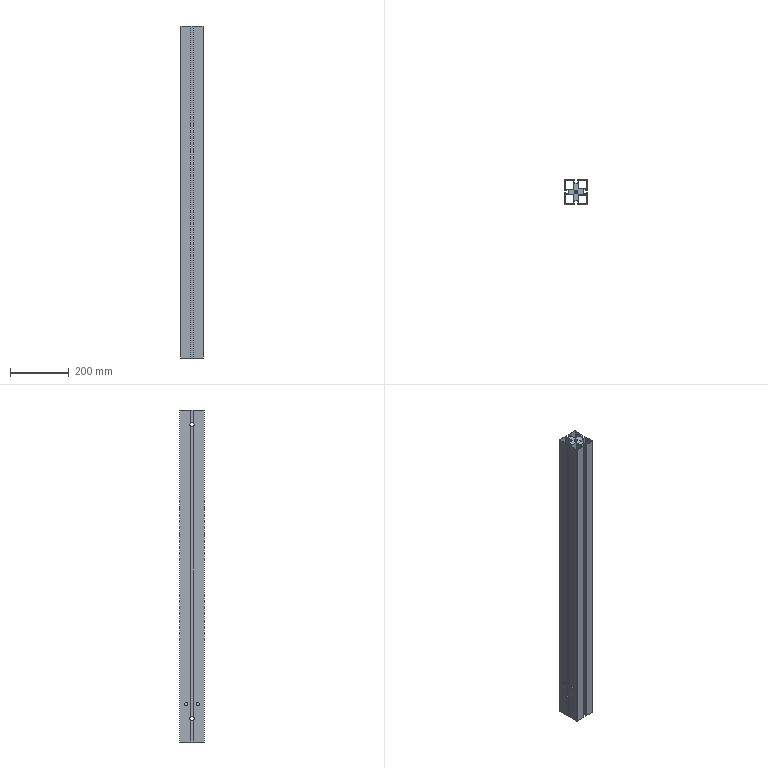Part | SolidWorks | features Cut 3, Extrusion 1, ICE 1 | 1 solid | 173 faces | box 76 x 85 x 1130 mm | volume 2230733 mm3 | plane 108 | cylinder 65 | commonest cylinder face diameters 1.3 x18 4 x16 10.2 x15 11 x8 1 x4 15 x2